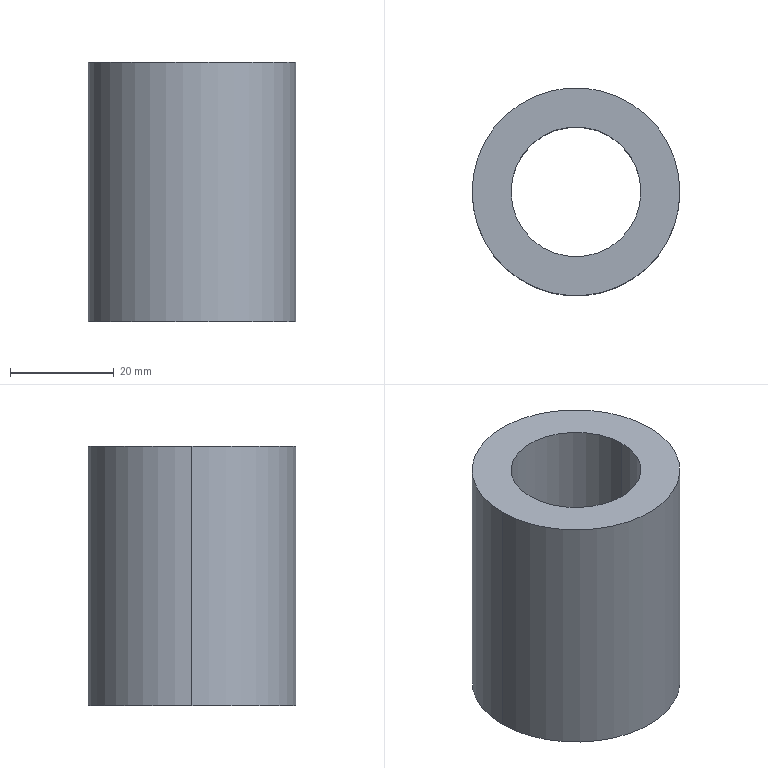Part | SolidWorks | features Extrusion 1 | 1 solid | 6 faces | box 40 x 40 x 50 mm | volume 38288 mm3 | cylinder 4 | plane 2 | commonest cylinder face diameters 25 x2 40 x2
STEP:
#1=CARTESIAN_POINT('',(-12.5,0.,25.));
#2=VERTEX_POINT('',#1);
#3=CARTESIAN_POINT('',(12.5,0.,25.));
#4=VERTEX_POINT('',#3);
#5=CARTESIAN_POINT('',(0.,0.,25.));
#6=DIRECTION('',(0.,0.,1.));
#7=DIRECTION('',(1.,0.,0.));
#8=AXIS2_PLACEMENT_3D('',#5,#6,#7);
#9=CIRCLE('',#8,12.5);
#10=EDGE_CURVE('',#2,#4,#9,.T.);
#11=ORIENTED_EDGE('',*,*,#10,.T.);
#12=CARTESIAN_POINT('',(12.5,0.,-25.));
#13=VERTEX_POINT('',#12);
#14=CARTESIAN_POINT('',(12.5,0.,25.));
#15=DIRECTION('',(0.,0.,-1.));
#16=VECTOR('',#15,1000.);
#17=LINE('',#14,#16);
#18=EDGE_CURVE('',#4,#13,#17,.T.);
#19=ORIENTED_EDGE('',*,*,#18,.T.);
#20=CARTESIAN_POINT('',(-12.5,0.,-25.));
#21=VERTEX_POINT('',#20);
#22=CARTESIAN_POINT('',(0.,0.,-25.));
#23=DIRECTION('',(0.,0.,1.));
#24=DIRECTION('',(1.,0.,0.));
#25=AXIS2_PLACEMENT_3D('',#22,#23,#24);
#26=CIRCLE('',#25,12.5);
#27=EDGE_CURVE('',#21,#13,#26,.T.);
#28=ORIENTED_EDGE('',*,*,#27,.F.);
#29=CARTESIAN_POINT('',(-12.5,0.,25.));
#30=DIRECTION('',(0.,0.,-1.));
#31=VECTOR('',#30,1000.);
#32=LINE('',#29,#31);
#33=EDGE_CURVE('',#2,#21,#32,.T.);
#34=ORIENTED_EDGE('',*,*,#33,.F.);
#35=EDGE_LOOP('',(#11,#19,#28,#34));
#36=FACE_OUTER_BOUND('',#35,.T.);
#37=CARTESIAN_POINT('',(0.,0.,25.));
#38=DIRECTION('',(0.,0.,-1.));
#39=DIRECTION('',(-1.,0.,0.));
#40=AXIS2_PLACEMENT_3D('',#37,#38,#39);
#41=CYLINDRICAL_SURFACE('',#40,12.5);
#42=ADVANCED_FACE('',(#36),#41,.F.);
#43=CARTESIAN_POINT('',(20.,0.,25.));
#44=VERTEX_POINT('',#43);
#45=CARTESIAN_POINT('',(-20.,0.,25.));
#46=VERTEX_POINT('',#45);
#47=CARTESIAN_POINT('',(0.,0.,25.));
#48=DIRECTION('',(0.,0.,1.));
#49=DIRECTION('',(1.,0.,0.));
#50=AXIS2_PLACEMENT_3D('',#47,#48,#49);
#51=CIRCLE('',#50,20.);
#52=EDGE_CURVE('',#44,#46,#51,.T.);
#53=ORIENTED_EDGE('',*,*,#52,.F.);
#54=CARTESIAN_POINT('',(20.,0.,-25.));
#55=VERTEX_POINT('',#54);
#56=CARTESIAN_POINT('',(20.,0.,25.));
#57=DIRECTION('',(0.,0.,-1.));
#58=VECTOR('',#57,1000.);
#59=LINE('',#56,#58);
#60=EDGE_CURVE('',#44,#55,#59,.T.);
#61=ORIENTED_EDGE('',*,*,#60,.T.);
#62=CARTESIAN_POINT('',(-20.,0.,-25.));
#63=VERTEX_POINT('',#62);
#64=CARTESIAN_POINT('',(0.,0.,-25.));
#65=DIRECTION('',(0.,0.,1.));
#66=DIRECTION('',(1.,0.,0.));
#67=AXIS2_PLACEMENT_3D('',#64,#65,#66);
#68=CIRCLE('',#67,20.);
#69=EDGE_CURVE('',#55,#63,#68,.T.);
#70=ORIENTED_EDGE('',*,*,#69,.T.);
#71=CARTESIAN_POINT('',(-20.,0.,25.));
#72=DIRECTION('',(0.,0.,-1.));
#73=VECTOR('',#72,1000.);
#74=LINE('',#71,#73);
#75=EDGE_CURVE('',#46,#63,#74,.T.);
#76=ORIENTED_EDGE('',*,*,#75,.F.);
#77=EDGE_LOOP('',(#53,#61,#70,#76));
#78=FACE_OUTER_BOUND('',#77,.T.);
#79=CARTESIAN_POINT('',(0.,0.,25.));
#80=DIRECTION('',(0.,0.,-1.));
#81=DIRECTION('',(-1.,0.,0.));
#82=AXIS2_PLACEMENT_3D('',#79,#80,#81);
#83=CYLINDRICAL_SURFACE('',#82,20.);
#84=ADVANCED_FACE('',(#78),#83,.T.);
#85=CARTESIAN_POINT('',(0.,0.,25.));
#86=DIRECTION('',(0.,0.,1.));
#87=DIRECTION('',(1.,0.,0.));
#88=AXIS2_PLACEMENT_3D('',#85,#86,#87);
#89=CIRCLE('',#88,20.);
#90=EDGE_CURVE('',#46,#44,#89,.T.);
#91=ORIENTED_EDGE('',*,*,#90,.T.);
#92=ORIENTED_EDGE('',*,*,#52,.T.);
#93=EDGE_LOOP('',(#91,#92));
#94=FACE_OUTER_BOUND('',#93,.T.);
#95=ORIENTED_EDGE('',*,*,#10,.F.);
#96=CARTESIAN_POINT('',(0.,0.,25.));
#97=DIRECTION('',(0.,0.,1.));
#98=DIRECTION('',(1.,0.,0.));
#99=AXIS2_PLACEMENT_3D('',#96,#97,#98);
#100=CIRCLE('',#99,12.5);
#101=EDGE_CURVE('',#4,#2,#100,.T.);
#102=ORIENTED_EDGE('',*,*,#101,.F.);
#103=EDGE_LOOP('',(#95,#102));
#104=FACE_BOUND('',#103,.T.);
#105=CARTESIAN_POINT('',(0.,0.,25.));
#106=DIRECTION('',(0.,0.,1.));
#107=DIRECTION('',(1.,0.,0.));
#108=AXIS2_PLACEMENT_3D('',#105,#106,#107);
#109=PLANE('',#108);
#110=ADVANCED_FACE('',(#94,#104),#109,.T.);
#111=CARTESIAN_POINT('',(0.,0.,-25.));
#112=DIRECTION('',(0.,0.,1.));
#113=DIRECTION('',(1.,0.,0.));
#114=AXIS2_PLACEMENT_3D('',#111,#112,#113);
#115=CIRCLE('',#114,20.);
#116=EDGE_CURVE('',#63,#55,#115,.T.);
#117=ORIENTED_EDGE('',*,*,#116,.F.);
#118=ORIENTED_EDGE('',*,*,#69,.F.);
#119=EDGE_LOOP('',(#117,#118));
#120=FACE_OUTER_BOUND('',#119,.T.);
#121=ORIENTED_EDGE('',*,*,#27,.T.);
#122=CARTESIAN_POINT('',(0.,0.,-25.));
#123=DIRECTION('',(0.,0.,1.));
#124=DIRECTION('',(1.,0.,0.));
#125=AXIS2_PLACEMENT_3D('',#122,#123,#124);
#126=CIRCLE('',#125,12.5);
#127=EDGE_CURVE('',#13,#21,#126,.T.);
#128=ORIENTED_EDGE('',*,*,#127,.T.);
#129=EDGE_LOOP('',(#121,#128));
#130=FACE_BOUND('',#129,.T.);
#131=CARTESIAN_POINT('',(0.,0.,-25.));
#132=DIRECTION('',(0.,0.,1.));
#133=DIRECTION('',(1.,0.,0.));
#134=AXIS2_PLACEMENT_3D('',#131,#132,#133);
#135=PLANE('',#134);
#136=ADVANCED_FACE('',(#120,#130),#135,.F.);
#137=ORIENTED_EDGE('',*,*,#60,.F.);
#138=ORIENTED_EDGE('',*,*,#90,.F.);
#139=ORIENTED_EDGE('',*,*,#75,.T.);
#140=ORIENTED_EDGE('',*,*,#116,.T.);
#141=EDGE_LOOP('',(#137,#138,#139,#140));
#142=FACE_OUTER_BOUND('',#141,.T.);
#143=CARTESIAN_POINT('',(0.,0.,25.));
#144=DIRECTION('',(0.,0.,-1.));
#145=DIRECTION('',(-1.,0.,0.));
#146=AXIS2_PLACEMENT_3D('',#143,#144,#145);
#147=CYLINDRICAL_SURFACE('',#146,20.);
#148=ADVANCED_FACE('',(#142),#147,.T.);
#149=ORIENTED_EDGE('',*,*,#18,.F.);
#150=ORIENTED_EDGE('',*,*,#101,.T.);
#151=ORIENTED_EDGE('',*,*,#33,.T.);
#152=ORIENTED_EDGE('',*,*,#127,.F.);
#153=EDGE_LOOP('',(#149,#150,#151,#152));
#154=FACE_OUTER_BOUND('',#153,.T.);
#155=CARTESIAN_POINT('',(0.,0.,25.));
#156=DIRECTION('',(0.,0.,-1.));
#157=DIRECTION('',(-1.,0.,0.));
#158=AXIS2_PLACEMENT_3D('',#155,#156,#157);
#159=CYLINDRICAL_SURFACE('',#158,12.5);
#160=ADVANCED_FACE('',(#154),#159,.F.);
#161=CLOSED_SHELL('',(#42,#84,#110,#136,#148,#160));
#162=MANIFOLD_SOLID_BREP('',#161);
#163=CARTESIAN_POINT('',(0.,0.,0.));
#164=DIRECTION('',(0.,0.,1.));
#165=DIRECTION('',(1.,0.,0.));
#166=AXIS2_PLACEMENT_3D('',#163,#164,#165);
#167=(LENGTH_UNIT()NAMED_UNIT(*)SI_UNIT(.MILLI.,.METRE.));
#168=UNCERTAINTY_MEASURE_WITH_UNIT(LENGTH_MEASURE(0.00001),#167,'','');
#169=(NAMED_UNIT(*)PLANE_ANGLE_UNIT()SI_UNIT($,.RADIAN.));
#170=(NAMED_UNIT(*)SI_UNIT($,.STERADIAN.)SOLID_ANGLE_UNIT());
#171=(GEOMETRIC_REPRESENTATION_CONTEXT(3)GLOBAL_UNCERTAINTY_ASSIGNED_CONTEXT((#168))GLOBAL_UNIT_ASSIGNED_CONTEXT((#167,#169,#170))REPRESENTATION_CONTEXT('',''));
#172=ADVANCED_BREP_SHAPE_REPRESENTATION('',(#162,#166),#171);